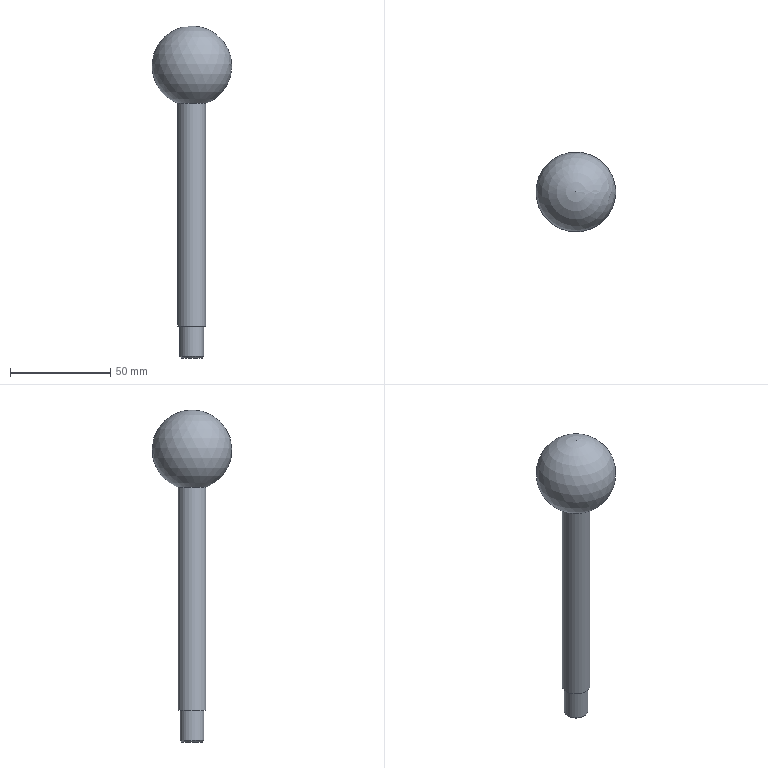Part | STEP file | YBQDJ-YY-9 | 1 solid | 6 faces | box 40 x 40 x 166 mm | volume 52339 mm3 | cylinder 2 | plane 2 | sphere 1 | cone 1 | commonest cylinder face diameters 12 x1 14 x1
STEP:
#1=CARTESIAN_POINT('',(0.,0.,0.));
#2=DIRECTION('',(0.,0.,1.));
#3=DIRECTION('',(1.,0.,0.));
#4=AXIS2_PLACEMENT_3D('',#1,#2,#3);
#5=CARTESIAN_POINT('',(223.5,305.,308.265));
#6=VERTEX_POINT('',#5);
#7=CARTESIAN_POINT('',(216.5,305.,308.265));
#8=DIRECTION('',(0.,0.,1.));
#9=DIRECTION('',(1.,0.,0.));
#10=AXIS2_PLACEMENT_3D('',#7,#8,#9);
#11=CIRCLE('',#10,7.);
#12=CARTESIAN_POINT('',(216.5,305.,285.));
#13=DIRECTION('',(0.,0.,-1.));
#14=DIRECTION('',(-1.,0.,0.));
#15=AXIS2_PLACEMENT_3D('',#12,#13,#14);
#16=CYLINDRICAL_SURFACE('',#15,7.);
#17=CARTESIAN_POINT('',(9.425,-23.265));
#18=DIRECTION('',(-1.,0.));
#19=VECTOR('',#18,1.);
#20=LINE('',#17,#19);
#21=(GEOMETRIC_REPRESENTATION_CONTEXT(2)PARAMETRIC_REPRESENTATION_CONTEXT()REPRESENTATION_CONTEXT('',''));
#22=DEFINITIONAL_REPRESENTATION('',(#20),#21);
#23=PCURVE('',#16,#22);
#24=CARTESIAN_POINT('',(216.5,305.,327.));
#25=DIRECTION('',(0.,0.,1.));
#26=DIRECTION('',(1.,0.,0.));
#27=AXIS2_PLACEMENT_3D('',#24,#25,#26);
#28=SPHERICAL_SURFACE('',#27,20.);
#29=CARTESIAN_POINT('',(0.,-1.213));
#30=CARTESIAN_POINT('',(0.0952,-1.213));
#31=CARTESIAN_POINT('',(0.2856,-1.213));
#32=CARTESIAN_POINT('',(0.5712,-1.213));
#33=CARTESIAN_POINT('',(0.8568,-1.213));
#34=CARTESIAN_POINT('',(1.142,-1.213));
#35=CARTESIAN_POINT('',(1.428,-1.213));
#36=CARTESIAN_POINT('',(1.714,-1.213));
#37=CARTESIAN_POINT('',(1.999,-1.213));
#38=CARTESIAN_POINT('',(2.285,-1.213));
#39=CARTESIAN_POINT('',(2.57,-1.213));
#40=CARTESIAN_POINT('',(2.856,-1.213));
#41=CARTESIAN_POINT('',(3.142,-1.213));
#42=CARTESIAN_POINT('',(3.427,-1.213));
#43=CARTESIAN_POINT('',(3.713,-1.213));
#44=CARTESIAN_POINT('',(3.998,-1.213));
#45=CARTESIAN_POINT('',(4.284,-1.213));
#46=CARTESIAN_POINT('',(4.57,-1.213));
#47=CARTESIAN_POINT('',(4.855,-1.213));
#48=CARTESIAN_POINT('',(5.141,-1.213));
#49=CARTESIAN_POINT('',(5.426,-1.213));
#50=CARTESIAN_POINT('',(5.712,-1.213));
#51=CARTESIAN_POINT('',(5.998,-1.213));
#52=CARTESIAN_POINT('',(6.188,-1.213));
#53=CARTESIAN_POINT('',(6.283,-1.213));
#54=B_SPLINE_CURVE_WITH_KNOTS('',3,(#29,#30,#31,#32,#33,#34,#35,#36,#37,#38,#39,#40,#41,#42,#43,#44,#45,#46,#47,#48,#49,#50,#51,#52,#53),.UNSPECIFIED.,.F.,.F.,(4,1,1,1,1,1,1,1,1,1,1,1,1,1,1,1,1,1,1,1,1,1,4),(0.,0.2856,0.5712,0.8568,1.142,1.428,1.714,1.999,2.285,2.57,2.856,3.142,3.427,3.713,3.998,4.284,4.57,4.855,5.141,5.426,5.712,5.998,6.283),.QUASI_UNIFORM_KNOTS.);
#55=(GEOMETRIC_REPRESENTATION_CONTEXT(2)PARAMETRIC_REPRESENTATION_CONTEXT()REPRESENTATION_CONTEXT('',''));
#56=DEFINITIONAL_REPRESENTATION('',(#54),#55);
#57=PCURVE('',#28,#56);
#58=SURFACE_CURVE('',#11,(#23,#57),.PCURVE_S1.);
#59=EDGE_CURVE('',#6,#6,#58,.T.);
#60=ORIENTED_EDGE('',*,*,#59,.F.);
#61=CARTESIAN_POINT('',(223.5,305.,197.));
#62=VERTEX_POINT('',#61);
#63=CARTESIAN_POINT('',(223.5,305.,308.265));
#64=CARTESIAN_POINT('',(223.5,305.,197.));
#65=B_SPLINE_CURVE_WITH_KNOTS('',1,(#63,#64),.UNSPECIFIED.,.F.,.F.,(2,2),(-23.265,88.),.PIECEWISE_BEZIER_KNOTS.);
#66=CARTESIAN_POINT('',(9.425,0.));
#67=DIRECTION('',(0.,1.));
#68=VECTOR('',#67,1.);
#69=LINE('',#66,#68);
#70=(GEOMETRIC_REPRESENTATION_CONTEXT(2)PARAMETRIC_REPRESENTATION_CONTEXT()REPRESENTATION_CONTEXT('',''));
#71=DEFINITIONAL_REPRESENTATION('',(#69),#70);
#72=PCURVE('',#16,#71);
#73=CARTESIAN_POINT('',(3.142,0.));
#74=DIRECTION('',(0.,1.));
#75=VECTOR('',#74,1.);
#76=LINE('',#73,#75);
#77=(GEOMETRIC_REPRESENTATION_CONTEXT(2)PARAMETRIC_REPRESENTATION_CONTEXT()REPRESENTATION_CONTEXT('',''));
#78=DEFINITIONAL_REPRESENTATION('',(#76),#77);
#79=PCURVE('',#16,#78);
#80=SEAM_CURVE('',#65,(#72,#79),.PCURVE_S1.);
#81=EDGE_CURVE('',#6,#62,#80,.T.);
#82=ORIENTED_EDGE('',*,*,#81,.T.);
#83=CARTESIAN_POINT('',(216.5,305.,197.));
#84=DIRECTION('',(0.,0.,1.));
#85=DIRECTION('',(1.,0.,0.));
#86=AXIS2_PLACEMENT_3D('',#83,#84,#85);
#87=CIRCLE('',#86,7.);
#88=CARTESIAN_POINT('',(9.425,88.));
#89=DIRECTION('',(-1.,0.));
#90=VECTOR('',#89,1.);
#91=LINE('',#88,#90);
#92=(GEOMETRIC_REPRESENTATION_CONTEXT(2)PARAMETRIC_REPRESENTATION_CONTEXT()REPRESENTATION_CONTEXT('',''));
#93=DEFINITIONAL_REPRESENTATION('',(#91),#92);
#94=PCURVE('',#16,#93);
#95=CARTESIAN_POINT('',(216.5,305.,197.));
#96=DIRECTION('',(0.,0.,1.));
#97=DIRECTION('',(1.,0.,0.));
#98=AXIS2_PLACEMENT_3D('',#95,#96,#97);
#99=PLANE('',#98);
#100=CARTESIAN_POINT('',(0.,0.));
#101=DIRECTION('',(1.,0.));
#102=AXIS2_PLACEMENT_2D('',#100,#101);
#103=CIRCLE('',#102,7.);
#104=(GEOMETRIC_REPRESENTATION_CONTEXT(2)PARAMETRIC_REPRESENTATION_CONTEXT()REPRESENTATION_CONTEXT('',''));
#105=DEFINITIONAL_REPRESENTATION('',(#103),#104);
#106=PCURVE('',#99,#105);
#107=SURFACE_CURVE('',#87,(#94,#106),.PCURVE_S1.);
#108=EDGE_CURVE('',#62,#62,#107,.T.);
#109=ORIENTED_EDGE('',*,*,#108,.T.);
#110=ORIENTED_EDGE('',*,*,#81,.F.);
#111=EDGE_LOOP('',(#60,#82,#109,#110));
#112=FACE_BOUND('',#111,.T.);
#113=ADVANCED_FACE('',(#112),#16,.T.);
#114=CARTESIAN_POINT('',(222.5,305.,197.));
#115=VERTEX_POINT('',#114);
#116=CARTESIAN_POINT('',(216.5,305.,197.));
#117=DIRECTION('',(0.,0.,1.));
#118=DIRECTION('',(1.,0.,0.));
#119=AXIS2_PLACEMENT_3D('',#116,#117,#118);
#120=CIRCLE('',#119,6.);
#121=CARTESIAN_POINT('',(0.,0.));
#122=DIRECTION('',(1.,0.));
#123=AXIS2_PLACEMENT_2D('',#121,#122);
#124=CIRCLE('',#123,6.);
#125=(GEOMETRIC_REPRESENTATION_CONTEXT(2)PARAMETRIC_REPRESENTATION_CONTEXT()REPRESENTATION_CONTEXT('',''));
#126=DEFINITIONAL_REPRESENTATION('',(#124),#125);
#127=PCURVE('',#99,#126);
#128=CARTESIAN_POINT('',(216.5,305.,181.));
#129=DIRECTION('',(0.,0.,1.));
#130=DIRECTION('',(1.,0.,0.));
#131=AXIS2_PLACEMENT_3D('',#128,#129,#130);
#132=CYLINDRICAL_SURFACE('',#131,6.);
#133=CARTESIAN_POINT('',(0.,16.));
#134=DIRECTION('',(1.,0.));
#135=VECTOR('',#134,1.);
#136=LINE('',#133,#135);
#137=(GEOMETRIC_REPRESENTATION_CONTEXT(2)PARAMETRIC_REPRESENTATION_CONTEXT()REPRESENTATION_CONTEXT('',''));
#138=DEFINITIONAL_REPRESENTATION('',(#136),#137);
#139=PCURVE('',#132,#138);
#140=SURFACE_CURVE('',#120,(#127,#139),.PCURVE_S1.);
#141=EDGE_CURVE('',#115,#115,#140,.T.);
#142=ORIENTED_EDGE('',*,*,#141,.T.);
#143=EDGE_LOOP('',(#142));
#144=FACE_BOUND('',#143,.T.);
#145=ORIENTED_EDGE('',*,*,#108,.F.);
#146=EDGE_LOOP('',(#145));
#147=FACE_BOUND('',#146,.T.);
#148=ADVANCED_FACE('',(#144,#147),#99,.F.);
#149=ORIENTED_EDGE('',*,*,#59,.T.);
#150=CARTESIAN_POINT('',(216.5,305.,347.));
#151=VERTEX_POINT('',#150);
#152=CARTESIAN_POINT('',(223.5,305.,308.265));
#153=CARTESIAN_POINT('',(229.295,305.,310.43));
#154=CARTESIAN_POINT('',(234.337,305.,314.613));
#155=CARTESIAN_POINT('',(237.823,305.,320.512));
#156=CARTESIAN_POINT('',(239.091,305.,327.456));
#157=CARTESIAN_POINT('',(237.822,305.,334.479));
#158=CARTESIAN_POINT('',(234.204,305.,340.541));
#159=CARTESIAN_POINT('',(228.873,305.,344.847));
#160=CARTESIAN_POINT('',(222.687,305.,347.));
#161=CARTESIAN_POINT('',(216.5,305.,347.));
#162=B_SPLINE_CURVE_WITH_KNOTS('',9,(#152,#153,#154,#155,#156,#157,#158,#159,#160,#161),.UNSPECIFIED.,.F.,.F.,(10,10),(-1.213,1.571),.PIECEWISE_BEZIER_KNOTS.);
#163=CARTESIAN_POINT('',(6.283,0.));
#164=DIRECTION('',(0.,1.));
#165=VECTOR('',#164,1.);
#166=LINE('',#163,#165);
#167=(GEOMETRIC_REPRESENTATION_CONTEXT(2)PARAMETRIC_REPRESENTATION_CONTEXT()REPRESENTATION_CONTEXT('',''));
#168=DEFINITIONAL_REPRESENTATION('',(#166),#167);
#169=PCURVE('',#28,#168);
#170=CARTESIAN_POINT('',(0.,0.));
#171=DIRECTION('',(0.,1.));
#172=VECTOR('',#171,1.);
#173=LINE('',#170,#172);
#174=(GEOMETRIC_REPRESENTATION_CONTEXT(2)PARAMETRIC_REPRESENTATION_CONTEXT()REPRESENTATION_CONTEXT('',''));
#175=DEFINITIONAL_REPRESENTATION('',(#173),#174);
#176=PCURVE('',#28,#175);
#177=SEAM_CURVE('',#162,(#169,#176),.PCURVE_S1.);
#178=EDGE_CURVE('',#6,#151,#177,.T.);
#179=ORIENTED_EDGE('',*,*,#178,.T.);
#180=ORIENTED_EDGE('',*,*,#178,.F.);
#181=EDGE_LOOP('',(#149,#179,#180));
#182=FACE_BOUND('',#181,.T.);
#183=ADVANCED_FACE('',(#182),#28,.T.);
#184=CARTESIAN_POINT('',(222.5,305.,181.75));
#185=VERTEX_POINT('',#184);
#186=CARTESIAN_POINT('',(216.5,305.,181.75));
#187=DIRECTION('',(0.,0.,1.));
#188=DIRECTION('',(1.,0.,0.));
#189=AXIS2_PLACEMENT_3D('',#186,#187,#188);
#190=CIRCLE('',#189,6.);
#191=CARTESIAN_POINT('',(0.,0.75));
#192=DIRECTION('',(1.,0.));
#193=VECTOR('',#192,1.);
#194=LINE('',#191,#193);
#195=(GEOMETRIC_REPRESENTATION_CONTEXT(2)PARAMETRIC_REPRESENTATION_CONTEXT()REPRESENTATION_CONTEXT('',''));
#196=DEFINITIONAL_REPRESENTATION('',(#194),#195);
#197=PCURVE('',#132,#196);
#198=CARTESIAN_POINT('',(216.5,305.,181.75));
#199=DIRECTION('',(0.,0.,1.));
#200=DIRECTION('',(1.,0.,0.));
#201=AXIS2_PLACEMENT_3D('',#198,#199,#200);
#202=CONICAL_SURFACE('',#201,6.,0.7854);
#203=CARTESIAN_POINT('',(0.,0.));
#204=DIRECTION('',(1.,0.));
#205=VECTOR('',#204,1.);
#206=LINE('',#203,#205);
#207=(GEOMETRIC_REPRESENTATION_CONTEXT(2)PARAMETRIC_REPRESENTATION_CONTEXT()REPRESENTATION_CONTEXT('',''));
#208=DEFINITIONAL_REPRESENTATION('',(#206),#207);
#209=PCURVE('',#202,#208);
#210=SURFACE_CURVE('',#190,(#197,#209),.PCURVE_S1.);
#211=EDGE_CURVE('',#185,#185,#210,.T.);
#212=ORIENTED_EDGE('',*,*,#211,.T.);
#213=CARTESIAN_POINT('',(222.5,305.,181.75));
#214=CARTESIAN_POINT('',(222.5,305.,197.));
#215=B_SPLINE_CURVE_WITH_KNOTS('',1,(#213,#214),.UNSPECIFIED.,.F.,.F.,(2,2),(0.75,16.),.PIECEWISE_BEZIER_KNOTS.);
#216=CARTESIAN_POINT('',(6.283,0.));
#217=DIRECTION('',(0.,1.));
#218=VECTOR('',#217,1.);
#219=LINE('',#216,#218);
#220=(GEOMETRIC_REPRESENTATION_CONTEXT(2)PARAMETRIC_REPRESENTATION_CONTEXT()REPRESENTATION_CONTEXT('',''));
#221=DEFINITIONAL_REPRESENTATION('',(#219),#220);
#222=PCURVE('',#132,#221);
#223=CARTESIAN_POINT('',(0.,0.));
#224=DIRECTION('',(0.,1.));
#225=VECTOR('',#224,1.);
#226=LINE('',#223,#225);
#227=(GEOMETRIC_REPRESENTATION_CONTEXT(2)PARAMETRIC_REPRESENTATION_CONTEXT()REPRESENTATION_CONTEXT('',''));
#228=DEFINITIONAL_REPRESENTATION('',(#226),#227);
#229=PCURVE('',#132,#228);
#230=SEAM_CURVE('',#215,(#222,#229),.PCURVE_S1.);
#231=EDGE_CURVE('',#185,#115,#230,.T.);
#232=ORIENTED_EDGE('',*,*,#231,.T.);
#233=ORIENTED_EDGE('',*,*,#141,.F.);
#234=ORIENTED_EDGE('',*,*,#231,.F.);
#235=EDGE_LOOP('',(#212,#232,#233,#234));
#236=FACE_BOUND('',#235,.T.);
#237=ADVANCED_FACE('',(#236),#132,.T.);
#238=CARTESIAN_POINT('',(221.75,305.,181.));
#239=VERTEX_POINT('',#238);
#240=CARTESIAN_POINT('',(216.5,305.,181.));
#241=DIRECTION('',(0.,0.,-1.));
#242=DIRECTION('',(1.,0.,0.));
#243=AXIS2_PLACEMENT_3D('',#240,#241,#242);
#244=CIRCLE('',#243,5.25);
#245=CARTESIAN_POINT('',(216.5,305.,181.));
#246=DIRECTION('',(0.,0.,1.));
#247=DIRECTION('',(1.,0.,0.));
#248=AXIS2_PLACEMENT_3D('',#245,#246,#247);
#249=PLANE('',#248);
#250=CARTESIAN_POINT('',(5.25,0.));
#251=CARTESIAN_POINT('',(5.25,-9.093));
#252=CARTESIAN_POINT('',(-2.625,-4.547));
#253=CARTESIAN_POINT('',(-10.5,0.));
#254=CARTESIAN_POINT('',(-2.625,4.547));
#255=CARTESIAN_POINT('',(5.25,9.093));
#256=CARTESIAN_POINT('',(5.25,0.));
#257=(BOUNDED_CURVE()B_SPLINE_CURVE(2,(#250,#251,#252,#253,#254,#255,#256),.UNSPECIFIED.,.T.,.F.)B_SPLINE_CURVE_WITH_KNOTS((1,2,2,2,2,1),(-2.094,0.,2.094,4.189,6.283,8.378),.UNSPECIFIED.)CURVE()GEOMETRIC_REPRESENTATION_ITEM()RATIONAL_B_SPLINE_CURVE((1.,0.5,1.,0.5,1.,0.5,1.))REPRESENTATION_ITEM(''));
#258=(GEOMETRIC_REPRESENTATION_CONTEXT(2)PARAMETRIC_REPRESENTATION_CONTEXT()REPRESENTATION_CONTEXT('',''));
#259=DEFINITIONAL_REPRESENTATION('',(#257),#258);
#260=PCURVE('',#249,#259);
#261=CARTESIAN_POINT('',(6.283,-0.75));
#262=DIRECTION('',(-1.,0.));
#263=VECTOR('',#262,1.);
#264=LINE('',#261,#263);
#265=(GEOMETRIC_REPRESENTATION_CONTEXT(2)PARAMETRIC_REPRESENTATION_CONTEXT()REPRESENTATION_CONTEXT('',''));
#266=DEFINITIONAL_REPRESENTATION('',(#264),#265);
#267=PCURVE('',#202,#266);
#268=SURFACE_CURVE('',#244,(#260,#267),.PCURVE_S1.);
#269=EDGE_CURVE('',#239,#239,#268,.T.);
#270=ORIENTED_EDGE('',*,*,#269,.T.);
#271=EDGE_LOOP('',(#270));
#272=FACE_BOUND('',#271,.T.);
#273=ADVANCED_FACE('',(#272),#249,.F.);
#274=ORIENTED_EDGE('',*,*,#269,.F.);
#275=CARTESIAN_POINT('',(221.75,305.,181.));
#276=CARTESIAN_POINT('',(222.5,305.,181.75));
#277=B_SPLINE_CURVE_WITH_KNOTS('',1,(#275,#276),.UNSPECIFIED.,.F.,.F.,(2,2),(-1.061,0.),.PIECEWISE_BEZIER_KNOTS.);
#278=CARTESIAN_POINT('',(6.283,0.));
#279=DIRECTION('',(0.,1.));
#280=VECTOR('',#279,1.);
#281=LINE('',#278,#280);
#282=(GEOMETRIC_REPRESENTATION_CONTEXT(2)PARAMETRIC_REPRESENTATION_CONTEXT()REPRESENTATION_CONTEXT('',''));
#283=DEFINITIONAL_REPRESENTATION('',(#281),#282);
#284=PCURVE('',#202,#283);
#285=CARTESIAN_POINT('',(0.,0.));
#286=DIRECTION('',(0.,1.));
#287=VECTOR('',#286,1.);
#288=LINE('',#285,#287);
#289=(GEOMETRIC_REPRESENTATION_CONTEXT(2)PARAMETRIC_REPRESENTATION_CONTEXT()REPRESENTATION_CONTEXT('',''));
#290=DEFINITIONAL_REPRESENTATION('',(#288),#289);
#291=PCURVE('',#202,#290);
#292=SEAM_CURVE('',#277,(#284,#291),.PCURVE_S1.);
#293=EDGE_CURVE('',#239,#185,#292,.T.);
#294=ORIENTED_EDGE('',*,*,#293,.T.);
#295=ORIENTED_EDGE('',*,*,#211,.F.);
#296=ORIENTED_EDGE('',*,*,#293,.F.);
#297=EDGE_LOOP('',(#274,#294,#295,#296));
#298=FACE_BOUND('',#297,.T.);
#299=ADVANCED_FACE('',(#298),#202,.T.);
#300=CLOSED_SHELL('',(#113,#148,#183,#237,#273,#299));
#301=MANIFOLD_SOLID_BREP('',#300);
#302=(LENGTH_UNIT()NAMED_UNIT(*)SI_UNIT(.MILLI.,.METRE.));
#303=UNCERTAINTY_MEASURE_WITH_UNIT(LENGTH_MEASURE(0.00001),#302,'','');
#304=(NAMED_UNIT(*)PLANE_ANGLE_UNIT()SI_UNIT($,.RADIAN.));
#305=(NAMED_UNIT(*)SI_UNIT($,.STERADIAN.)SOLID_ANGLE_UNIT());
#306=(GEOMETRIC_REPRESENTATION_CONTEXT(3)GLOBAL_UNCERTAINTY_ASSIGNED_CONTEXT((#303))GLOBAL_UNIT_ASSIGNED_CONTEXT((#302,#304,#305))REPRESENTATION_CONTEXT('',''));
#307=ADVANCED_BREP_SHAPE_REPRESENTATION('',(#4,#301),#306);